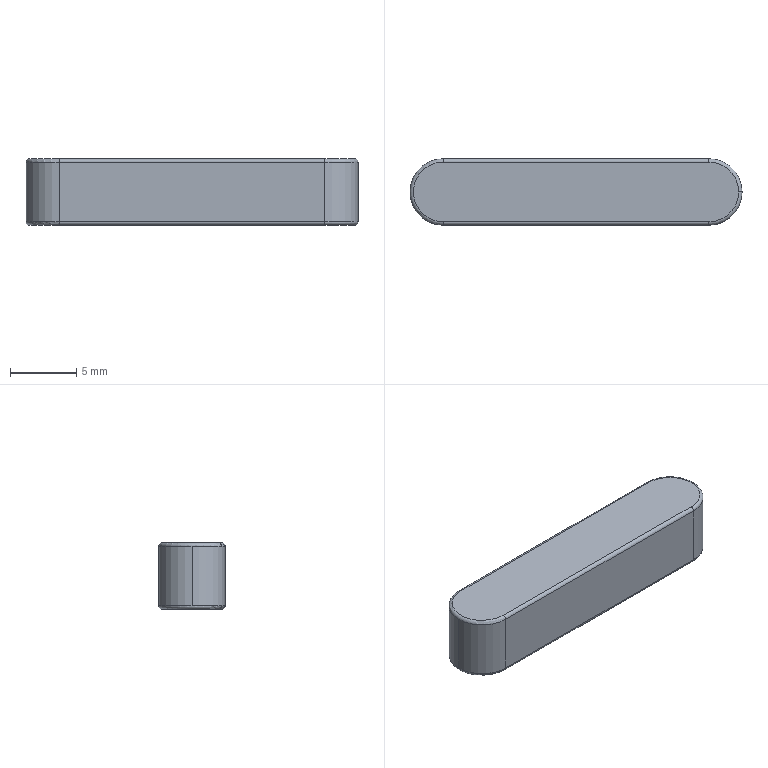Part | SolidWorks | features Extrusion 1, Fillet 1 | 1 solid | 17 faces | box 25 x 5 x 5 mm | volume 596.69 mm3 | cylinder 7 | torus 6 | plane 4 | commonest cylinder face diameters 0.5 x4 5 x3
STEP:
#1=CARTESIAN_POINT('',(12.25,0.,0.));
#2=VERTEX_POINT('',#1);
#3=CARTESIAN_POINT('',(10.,-2.25,0.));
#4=VERTEX_POINT('',#3);
#5=CARTESIAN_POINT('',(10.,0.,0.));
#6=DIRECTION('',(0.,0.,-1.));
#7=DIRECTION('',(1.,0.,0.));
#8=AXIS2_PLACEMENT_3D('',#5,#6,#7);
#9=CIRCLE('',#8,2.25);
#10=EDGE_CURVE('',#2,#4,#9,.T.);
#11=ORIENTED_EDGE('',*,*,#10,.F.);
#12=CARTESIAN_POINT('',(12.5,0.,0.25));
#13=VERTEX_POINT('',#12);
#14=CARTESIAN_POINT('',(12.25,0.,0.25));
#15=DIRECTION('',(0.,-1.,0.));
#16=DIRECTION('',(0.,0.,-1.));
#17=AXIS2_PLACEMENT_3D('',#14,#15,#16);
#18=CIRCLE('',#17,0.25);
#19=EDGE_CURVE('',#2,#13,#18,.T.);
#20=ORIENTED_EDGE('',*,*,#19,.T.);
#21=CARTESIAN_POINT('',(10.,-2.5,0.25));
#22=VERTEX_POINT('',#21);
#23=CARTESIAN_POINT('',(10.,0.,0.25));
#24=DIRECTION('',(0.,0.,1.));
#25=DIRECTION('',(1.,0.,0.));
#26=AXIS2_PLACEMENT_3D('',#23,#24,#25);
#27=CIRCLE('',#26,2.5);
#28=EDGE_CURVE('',#22,#13,#27,.T.);
#29=ORIENTED_EDGE('',*,*,#28,.F.);
#30=CARTESIAN_POINT('',(10.,-2.25,0.25));
#31=DIRECTION('',(1.,0.,0.));
#32=DIRECTION('',(0.,0.,-1.));
#33=AXIS2_PLACEMENT_3D('',#30,#31,#32);
#34=CIRCLE('',#33,0.25);
#35=EDGE_CURVE('',#22,#4,#34,.T.);
#36=ORIENTED_EDGE('',*,*,#35,.T.);
#37=EDGE_LOOP('',(#11,#20,#29,#36));
#38=FACE_OUTER_BOUND('',#37,.T.);
#39=CARTESIAN_POINT('',(10.,0.,0.25));
#40=DIRECTION('',(0.,0.,1.));
#41=DIRECTION('',(1.,0.,0.));
#42=AXIS2_PLACEMENT_3D('',#39,#40,#41);
#43=TOROIDAL_SURFACE('',#42,2.25,0.25);
#44=ADVANCED_FACE('',(#38),#43,.T.);
#45=CARTESIAN_POINT('',(12.5,0.,4.75));
#46=VERTEX_POINT('',#45);
#47=CARTESIAN_POINT('',(10.,-2.5,4.75));
#48=VERTEX_POINT('',#47);
#49=CARTESIAN_POINT('',(10.,0.,4.75));
#50=DIRECTION('',(0.,0.,-1.));
#51=DIRECTION('',(1.,0.,0.));
#52=AXIS2_PLACEMENT_3D('',#49,#50,#51);
#53=CIRCLE('',#52,2.5);
#54=EDGE_CURVE('',#46,#48,#53,.T.);
#55=ORIENTED_EDGE('',*,*,#54,.F.);
#56=CARTESIAN_POINT('',(12.25,0.,5.));
#57=VERTEX_POINT('',#56);
#58=CARTESIAN_POINT('',(12.25,0.,4.75));
#59=DIRECTION('',(0.,-1.,0.));
#60=DIRECTION('',(0.,0.,-1.));
#61=AXIS2_PLACEMENT_3D('',#58,#59,#60);
#62=CIRCLE('',#61,0.25);
#63=EDGE_CURVE('',#46,#57,#62,.T.);
#64=ORIENTED_EDGE('',*,*,#63,.T.);
#65=CARTESIAN_POINT('',(10.,-2.25,5.));
#66=VERTEX_POINT('',#65);
#67=CARTESIAN_POINT('',(10.,0.,5.));
#68=DIRECTION('',(0.,0.,1.));
#69=DIRECTION('',(1.,0.,0.));
#70=AXIS2_PLACEMENT_3D('',#67,#68,#69);
#71=CIRCLE('',#70,2.25);
#72=EDGE_CURVE('',#66,#57,#71,.T.);
#73=ORIENTED_EDGE('',*,*,#72,.F.);
#74=CARTESIAN_POINT('',(10.,-2.25,4.75));
#75=DIRECTION('',(1.,0.,0.));
#76=DIRECTION('',(0.,0.,-1.));
#77=AXIS2_PLACEMENT_3D('',#74,#75,#76);
#78=CIRCLE('',#77,0.25);
#79=EDGE_CURVE('',#66,#48,#78,.T.);
#80=ORIENTED_EDGE('',*,*,#79,.T.);
#81=EDGE_LOOP('',(#55,#64,#73,#80));
#82=FACE_OUTER_BOUND('',#81,.T.);
#83=CARTESIAN_POINT('',(10.,0.,4.75));
#84=DIRECTION('',(0.,0.,1.));
#85=DIRECTION('',(1.,0.,0.));
#86=AXIS2_PLACEMENT_3D('',#83,#84,#85);
#87=TOROIDAL_SURFACE('',#86,2.25,0.25);
#88=ADVANCED_FACE('',(#82),#87,.T.);
#89=CARTESIAN_POINT('',(-10.,-2.5,4.75));
#90=VERTEX_POINT('',#89);
#91=CARTESIAN_POINT('',(-12.5,0.,4.75));
#92=VERTEX_POINT('',#91);
#93=CARTESIAN_POINT('',(-10.,0.,4.75));
#94=DIRECTION('',(0.,0.,-1.));
#95=DIRECTION('',(1.,0.,0.));
#96=AXIS2_PLACEMENT_3D('',#93,#94,#95);
#97=CIRCLE('',#96,2.5);
#98=EDGE_CURVE('',#90,#92,#97,.T.);
#99=ORIENTED_EDGE('',*,*,#98,.T.);
#100=CARTESIAN_POINT('',(-12.5,0.,0.25));
#101=VERTEX_POINT('',#100);
#102=CARTESIAN_POINT('',(-12.5,0.,5.));
#103=DIRECTION('',(0.,0.,-1.));
#104=VECTOR('',#103,1000.);
#105=LINE('',#102,#104);
#106=EDGE_CURVE('',#92,#101,#105,.T.);
#107=ORIENTED_EDGE('',*,*,#106,.T.);
#108=CARTESIAN_POINT('',(-10.,-2.5,0.25));
#109=VERTEX_POINT('',#108);
#110=CARTESIAN_POINT('',(-10.,0.,0.25));
#111=DIRECTION('',(0.,0.,1.));
#112=DIRECTION('',(1.,0.,0.));
#113=AXIS2_PLACEMENT_3D('',#110,#111,#112);
#114=CIRCLE('',#113,2.5);
#115=EDGE_CURVE('',#101,#109,#114,.T.);
#116=ORIENTED_EDGE('',*,*,#115,.T.);
#117=CARTESIAN_POINT('',(-10.,-2.5,5.));
#118=DIRECTION('',(0.,0.,-1.));
#119=VECTOR('',#118,1000.);
#120=LINE('',#117,#119);
#121=EDGE_CURVE('',#90,#109,#120,.T.);
#122=ORIENTED_EDGE('',*,*,#121,.F.);
#123=EDGE_LOOP('',(#99,#107,#116,#122));
#124=FACE_OUTER_BOUND('',#123,.T.);
#125=CARTESIAN_POINT('',(-10.,0.,5.));
#126=DIRECTION('',(0.,0.,-1.));
#127=DIRECTION('',(-1.,0.,0.));
#128=AXIS2_PLACEMENT_3D('',#125,#126,#127);
#129=CYLINDRICAL_SURFACE('',#128,2.5);
#130=ADVANCED_FACE('',(#124),#129,.T.);
#131=ORIENTED_EDGE('',*,*,#106,.F.);
#132=CARTESIAN_POINT('',(-10.,2.5,4.75));
#133=VERTEX_POINT('',#132);
#134=CARTESIAN_POINT('',(-10.,0.,4.75));
#135=DIRECTION('',(0.,0.,-1.));
#136=DIRECTION('',(1.,0.,0.));
#137=AXIS2_PLACEMENT_3D('',#134,#135,#136);
#138=CIRCLE('',#137,2.5);
#139=EDGE_CURVE('',#92,#133,#138,.T.);
#140=ORIENTED_EDGE('',*,*,#139,.T.);
#141=CARTESIAN_POINT('',(-10.,2.5,0.25));
#142=VERTEX_POINT('',#141);
#143=CARTESIAN_POINT('',(-10.,2.5,5.));
#144=DIRECTION('',(0.,0.,-1.));
#145=VECTOR('',#144,1000.);
#146=LINE('',#143,#145);
#147=EDGE_CURVE('',#133,#142,#146,.T.);
#148=ORIENTED_EDGE('',*,*,#147,.T.);
#149=CARTESIAN_POINT('',(-10.,0.,0.25));
#150=DIRECTION('',(0.,0.,1.));
#151=DIRECTION('',(1.,0.,0.));
#152=AXIS2_PLACEMENT_3D('',#149,#150,#151);
#153=CIRCLE('',#152,2.5);
#154=EDGE_CURVE('',#142,#101,#153,.T.);
#155=ORIENTED_EDGE('',*,*,#154,.T.);
#156=EDGE_LOOP('',(#131,#140,#148,#155));
#157=FACE_OUTER_BOUND('',#156,.T.);
#158=CARTESIAN_POINT('',(-10.,0.,5.));
#159=DIRECTION('',(0.,0.,-1.));
#160=DIRECTION('',(-1.,0.,0.));
#161=AXIS2_PLACEMENT_3D('',#158,#159,#160);
#162=CYLINDRICAL_SURFACE('',#161,2.5);
#163=ADVANCED_FACE('',(#157),#162,.T.);
#164=CARTESIAN_POINT('',(10.,-2.5,5.));
#165=DIRECTION('',(0.,0.,-1.));
#166=VECTOR('',#165,1000.);
#167=LINE('',#164,#166);
#168=EDGE_CURVE('',#48,#22,#167,.T.);
#169=ORIENTED_EDGE('',*,*,#168,.F.);
#170=CARTESIAN_POINT('',(-10.,-2.5,4.75));
#171=DIRECTION('',(-1.,0.,0.));
#172=VECTOR('',#171,1000.);
#173=LINE('',#170,#172);
#174=EDGE_CURVE('',#48,#90,#173,.T.);
#175=ORIENTED_EDGE('',*,*,#174,.T.);
#176=ORIENTED_EDGE('',*,*,#121,.T.);
#177=CARTESIAN_POINT('',(-10.,-2.5,0.25));
#178=DIRECTION('',(1.,0.,0.));
#179=VECTOR('',#178,1000.);
#180=LINE('',#177,#179);
#181=EDGE_CURVE('',#109,#22,#180,.T.);
#182=ORIENTED_EDGE('',*,*,#181,.T.);
#183=EDGE_LOOP('',(#169,#175,#176,#182));
#184=FACE_OUTER_BOUND('',#183,.T.);
#185=CARTESIAN_POINT('',(-10.,-2.5,5.));
#186=DIRECTION('',(0.,1.,0.));
#187=DIRECTION('',(0.,0.,1.));
#188=AXIS2_PLACEMENT_3D('',#185,#186,#187);
#189=PLANE('',#188);
#190=ADVANCED_FACE('',(#184),#189,.F.);
#191=CARTESIAN_POINT('',(10.,2.5,4.75));
#192=VERTEX_POINT('',#191);
#193=CARTESIAN_POINT('',(10.,2.5,0.25));
#194=VERTEX_POINT('',#193);
#195=CARTESIAN_POINT('',(10.,2.5,5.));
#196=DIRECTION('',(0.,0.,-1.));
#197=VECTOR('',#196,1000.);
#198=LINE('',#195,#197);
#199=EDGE_CURVE('',#192,#194,#198,.T.);
#200=ORIENTED_EDGE('',*,*,#199,.F.);
#201=CARTESIAN_POINT('',(10.,0.,4.75));
#202=DIRECTION('',(0.,0.,-1.));
#203=DIRECTION('',(1.,0.,0.));
#204=AXIS2_PLACEMENT_3D('',#201,#202,#203);
#205=CIRCLE('',#204,2.5);
#206=EDGE_CURVE('',#192,#46,#205,.T.);
#207=ORIENTED_EDGE('',*,*,#206,.T.);
#208=ORIENTED_EDGE('',*,*,#54,.T.);
#209=ORIENTED_EDGE('',*,*,#168,.T.);
#210=ORIENTED_EDGE('',*,*,#28,.T.);
#211=CARTESIAN_POINT('',(10.,0.,0.25));
#212=DIRECTION('',(0.,0.,1.));
#213=DIRECTION('',(1.,0.,0.));
#214=AXIS2_PLACEMENT_3D('',#211,#212,#213);
#215=CIRCLE('',#214,2.5);
#216=EDGE_CURVE('',#13,#194,#215,.T.);
#217=ORIENTED_EDGE('',*,*,#216,.T.);
#218=EDGE_LOOP('',(#200,#207,#208,#209,#210,#217));
#219=FACE_OUTER_BOUND('',#218,.T.);
#220=CARTESIAN_POINT('',(10.,0.,5.));
#221=DIRECTION('',(0.,0.,-1.));
#222=DIRECTION('',(-1.,0.,0.));
#223=AXIS2_PLACEMENT_3D('',#220,#221,#222);
#224=CYLINDRICAL_SURFACE('',#223,2.5);
#225=ADVANCED_FACE('',(#219),#224,.T.);
#226=ORIENTED_EDGE('',*,*,#147,.F.);
#227=CARTESIAN_POINT('',(10.,2.5,4.75));
#228=DIRECTION('',(1.,0.,0.));
#229=VECTOR('',#228,1000.);
#230=LINE('',#227,#229);
#231=EDGE_CURVE('',#133,#192,#230,.T.);
#232=ORIENTED_EDGE('',*,*,#231,.T.);
#233=ORIENTED_EDGE('',*,*,#199,.T.);
#234=CARTESIAN_POINT('',(-10.,2.5,0.25));
#235=DIRECTION('',(-1.,0.,0.));
#236=VECTOR('',#235,1000.);
#237=LINE('',#234,#236);
#238=EDGE_CURVE('',#194,#142,#237,.T.);
#239=ORIENTED_EDGE('',*,*,#238,.T.);
#240=EDGE_LOOP('',(#226,#232,#233,#239));
#241=FACE_OUTER_BOUND('',#240,.T.);
#242=CARTESIAN_POINT('',(-10.,2.5,5.));
#243=DIRECTION('',(0.,-1.,0.));
#244=DIRECTION('',(0.,0.,-1.));
#245=AXIS2_PLACEMENT_3D('',#242,#243,#244);
#246=PLANE('',#245);
#247=ADVANCED_FACE('',(#241),#246,.F.);
#248=CARTESIAN_POINT('',(-10.,-2.25,5.));
#249=VERTEX_POINT('',#248);
#250=CARTESIAN_POINT('',(10.,-2.25,5.));
#251=DIRECTION('',(1.,0.,0.));
#252=VECTOR('',#251,1000.);
#253=LINE('',#250,#252);
#254=EDGE_CURVE('',#249,#66,#253,.T.);
#255=ORIENTED_EDGE('',*,*,#254,.T.);
#256=ORIENTED_EDGE('',*,*,#72,.T.);
#257=CARTESIAN_POINT('',(10.,2.25,5.));
#258=VERTEX_POINT('',#257);
#259=CARTESIAN_POINT('',(10.,0.,5.));
#260=DIRECTION('',(0.,0.,1.));
#261=DIRECTION('',(1.,0.,0.));
#262=AXIS2_PLACEMENT_3D('',#259,#260,#261);
#263=CIRCLE('',#262,2.25);
#264=EDGE_CURVE('',#57,#258,#263,.T.);
#265=ORIENTED_EDGE('',*,*,#264,.T.);
#266=CARTESIAN_POINT('',(-10.,2.25,5.));
#267=VERTEX_POINT('',#266);
#268=CARTESIAN_POINT('',(-10.,2.25,5.));
#269=DIRECTION('',(-1.,0.,0.));
#270=VECTOR('',#269,1000.);
#271=LINE('',#268,#270);
#272=EDGE_CURVE('',#258,#267,#271,.T.);
#273=ORIENTED_EDGE('',*,*,#272,.T.);
#274=CARTESIAN_POINT('',(-10.,0.,5.));
#275=DIRECTION('',(0.,0.,1.));
#276=DIRECTION('',(1.,0.,0.));
#277=AXIS2_PLACEMENT_3D('',#274,#275,#276);
#278=CIRCLE('',#277,2.25);
#279=EDGE_CURVE('',#267,#249,#278,.T.);
#280=ORIENTED_EDGE('',*,*,#279,.T.);
#281=EDGE_LOOP('',(#255,#256,#265,#273,#280));
#282=FACE_OUTER_BOUND('',#281,.T.);
#283=CARTESIAN_POINT('',(-10.,0.,5.));
#284=DIRECTION('',(0.,0.,1.));
#285=DIRECTION('',(1.,0.,0.));
#286=AXIS2_PLACEMENT_3D('',#283,#284,#285);
#287=PLANE('',#286);
#288=ADVANCED_FACE('',(#282),#287,.T.);
#289=CARTESIAN_POINT('',(-10.,2.25,0.));
#290=VERTEX_POINT('',#289);
#291=CARTESIAN_POINT('',(10.,2.25,0.));
#292=VERTEX_POINT('',#291);
#293=CARTESIAN_POINT('',(-10.,2.25,0.));
#294=DIRECTION('',(1.,0.,0.));
#295=VECTOR('',#294,1000.);
#296=LINE('',#293,#295);
#297=EDGE_CURVE('',#290,#292,#296,.T.);
#298=ORIENTED_EDGE('',*,*,#297,.T.);
#299=CARTESIAN_POINT('',(10.,0.,0.));
#300=DIRECTION('',(0.,0.,-1.));
#301=DIRECTION('',(1.,0.,0.));
#302=AXIS2_PLACEMENT_3D('',#299,#300,#301);
#303=CIRCLE('',#302,2.25);
#304=EDGE_CURVE('',#292,#2,#303,.T.);
#305=ORIENTED_EDGE('',*,*,#304,.T.);
#306=ORIENTED_EDGE('',*,*,#10,.T.);
#307=CARTESIAN_POINT('',(-10.,-2.25,0.));
#308=VERTEX_POINT('',#307);
#309=CARTESIAN_POINT('',(-10.,-2.25,0.));
#310=DIRECTION('',(-1.,0.,0.));
#311=VECTOR('',#310,1000.);
#312=LINE('',#309,#311);
#313=EDGE_CURVE('',#4,#308,#312,.T.);
#314=ORIENTED_EDGE('',*,*,#313,.T.);
#315=CARTESIAN_POINT('',(-10.,0.,0.));
#316=DIRECTION('',(0.,0.,-1.));
#317=DIRECTION('',(1.,0.,0.));
#318=AXIS2_PLACEMENT_3D('',#315,#316,#317);
#319=CIRCLE('',#318,2.25);
#320=EDGE_CURVE('',#308,#290,#319,.T.);
#321=ORIENTED_EDGE('',*,*,#320,.T.);
#322=EDGE_LOOP('',(#298,#305,#306,#314,#321));
#323=FACE_OUTER_BOUND('',#322,.T.);
#324=CARTESIAN_POINT('',(-10.,0.,0.));
#325=DIRECTION('',(0.,0.,1.));
#326=DIRECTION('',(1.,0.,0.));
#327=AXIS2_PLACEMENT_3D('',#324,#325,#326);
#328=PLANE('',#327);
#329=ADVANCED_FACE('',(#323),#328,.F.);
#330=CARTESIAN_POINT('',(-10.,2.25,4.75));
#331=DIRECTION('',(1.,0.,0.));
#332=DIRECTION('',(0.,0.,-1.));
#333=AXIS2_PLACEMENT_3D('',#330,#331,#332);
#334=CIRCLE('',#333,0.25);
#335=EDGE_CURVE('',#133,#267,#334,.T.);
#336=ORIENTED_EDGE('',*,*,#335,.F.);
#337=ORIENTED_EDGE('',*,*,#139,.F.);
#338=ORIENTED_EDGE('',*,*,#98,.F.);
#339=CARTESIAN_POINT('',(-10.,-2.25,4.75));
#340=DIRECTION('',(1.,0.,0.));
#341=DIRECTION('',(0.,0.,-1.));
#342=AXIS2_PLACEMENT_3D('',#339,#340,#341);
#343=CIRCLE('',#342,0.25);
#344=EDGE_CURVE('',#249,#90,#343,.T.);
#345=ORIENTED_EDGE('',*,*,#344,.F.);
#346=ORIENTED_EDGE('',*,*,#279,.F.);
#347=EDGE_LOOP('',(#336,#337,#338,#345,#346));
#348=FACE_OUTER_BOUND('',#347,.T.);
#349=CARTESIAN_POINT('',(-10.,0.,4.75));
#350=DIRECTION('',(0.,0.,1.));
#351=DIRECTION('',(1.,0.,0.));
#352=AXIS2_PLACEMENT_3D('',#349,#350,#351);
#353=TOROIDAL_SURFACE('',#352,2.25,0.25);
#354=ADVANCED_FACE('',(#348),#353,.T.);
#355=ORIENTED_EDGE('',*,*,#344,.T.);
#356=ORIENTED_EDGE('',*,*,#174,.F.);
#357=ORIENTED_EDGE('',*,*,#79,.F.);
#358=ORIENTED_EDGE('',*,*,#254,.F.);
#359=EDGE_LOOP('',(#355,#356,#357,#358));
#360=FACE_OUTER_BOUND('',#359,.T.);
#361=CARTESIAN_POINT('',(-10.,-2.25,4.75));
#362=DIRECTION('',(-1.,0.,0.));
#363=DIRECTION('',(0.,0.,1.));
#364=AXIS2_PLACEMENT_3D('',#361,#362,#363);
#365=CYLINDRICAL_SURFACE('',#364,0.25);
#366=ADVANCED_FACE('',(#360),#365,.T.);
#367=ORIENTED_EDGE('',*,*,#335,.T.);
#368=ORIENTED_EDGE('',*,*,#272,.F.);
#369=CARTESIAN_POINT('',(10.,2.25,4.75));
#370=DIRECTION('',(1.,0.,0.));
#371=DIRECTION('',(0.,0.,-1.));
#372=AXIS2_PLACEMENT_3D('',#369,#370,#371);
#373=CIRCLE('',#372,0.25);
#374=EDGE_CURVE('',#192,#258,#373,.T.);
#375=ORIENTED_EDGE('',*,*,#374,.F.);
#376=ORIENTED_EDGE('',*,*,#231,.F.);
#377=EDGE_LOOP('',(#367,#368,#375,#376));
#378=FACE_OUTER_BOUND('',#377,.T.);
#379=CARTESIAN_POINT('',(-10.,2.25,4.75));
#380=DIRECTION('',(1.,0.,0.));
#381=DIRECTION('',(0.,0.,-1.));
#382=AXIS2_PLACEMENT_3D('',#379,#380,#381);
#383=CYLINDRICAL_SURFACE('',#382,0.25);
#384=ADVANCED_FACE('',(#378),#383,.T.);
#385=ORIENTED_EDGE('',*,*,#63,.F.);
#386=ORIENTED_EDGE('',*,*,#206,.F.);
#387=ORIENTED_EDGE('',*,*,#374,.T.);
#388=ORIENTED_EDGE('',*,*,#264,.F.);
#389=EDGE_LOOP('',(#385,#386,#387,#388));
#390=FACE_OUTER_BOUND('',#389,.T.);
#391=CARTESIAN_POINT('',(10.,0.,4.75));
#392=DIRECTION('',(0.,0.,1.));
#393=DIRECTION('',(1.,0.,0.));
#394=AXIS2_PLACEMENT_3D('',#391,#392,#393);
#395=TOROIDAL_SURFACE('',#394,2.25,0.25);
#396=ADVANCED_FACE('',(#390),#395,.T.);
#397=CARTESIAN_POINT('',(-10.,2.25,0.25));
#398=DIRECTION('',(1.,0.,0.));
#399=DIRECTION('',(0.,0.,-1.));
#400=AXIS2_PLACEMENT_3D('',#397,#398,#399);
#401=CIRCLE('',#400,0.25);
#402=EDGE_CURVE('',#290,#142,#401,.T.);
#403=ORIENTED_EDGE('',*,*,#402,.F.);
#404=ORIENTED_EDGE('',*,*,#320,.F.);
#405=CARTESIAN_POINT('',(-10.,-2.25,0.25));
#406=DIRECTION('',(1.,0.,0.));
#407=DIRECTION('',(0.,0.,-1.));
#408=AXIS2_PLACEMENT_3D('',#405,#406,#407);
#409=CIRCLE('',#408,0.25);
#410=EDGE_CURVE('',#109,#308,#409,.T.);
#411=ORIENTED_EDGE('',*,*,#410,.F.);
#412=ORIENTED_EDGE('',*,*,#115,.F.);
#413=ORIENTED_EDGE('',*,*,#154,.F.);
#414=EDGE_LOOP('',(#403,#404,#411,#412,#413));
#415=FACE_OUTER_BOUND('',#414,.T.);
#416=CARTESIAN_POINT('',(-10.,0.,0.25));
#417=DIRECTION('',(0.,0.,1.));
#418=DIRECTION('',(1.,0.,0.));
#419=AXIS2_PLACEMENT_3D('',#416,#417,#418);
#420=TOROIDAL_SURFACE('',#419,2.25,0.25);
#421=ADVANCED_FACE('',(#415),#420,.T.);
#422=ORIENTED_EDGE('',*,*,#410,.T.);
#423=ORIENTED_EDGE('',*,*,#313,.F.);
#424=ORIENTED_EDGE('',*,*,#35,.F.);
#425=ORIENTED_EDGE('',*,*,#181,.F.);
#426=EDGE_LOOP('',(#422,#423,#424,#425));
#427=FACE_OUTER_BOUND('',#426,.T.);
#428=CARTESIAN_POINT('',(-10.,-2.25,0.25));
#429=DIRECTION('',(1.,0.,0.));
#430=DIRECTION('',(0.,0.,-1.));
#431=AXIS2_PLACEMENT_3D('',#428,#429,#430);
#432=CYLINDRICAL_SURFACE('',#431,0.25);
#433=ADVANCED_FACE('',(#427),#432,.T.);
#434=ORIENTED_EDGE('',*,*,#402,.T.);
#435=ORIENTED_EDGE('',*,*,#238,.F.);
#436=CARTESIAN_POINT('',(10.,2.25,0.25));
#437=DIRECTION('',(1.,0.,0.));
#438=DIRECTION('',(0.,0.,-1.));
#439=AXIS2_PLACEMENT_3D('',#436,#437,#438);
#440=CIRCLE('',#439,0.25);
#441=EDGE_CURVE('',#292,#194,#440,.T.);
#442=ORIENTED_EDGE('',*,*,#441,.F.);
#443=ORIENTED_EDGE('',*,*,#297,.F.);
#444=EDGE_LOOP('',(#434,#435,#442,#443));
#445=FACE_OUTER_BOUND('',#444,.T.);
#446=CARTESIAN_POINT('',(-10.,2.25,0.25));
#447=DIRECTION('',(-1.,0.,0.));
#448=DIRECTION('',(0.,0.,1.));
#449=AXIS2_PLACEMENT_3D('',#446,#447,#448);
#450=CYLINDRICAL_SURFACE('',#449,0.25);
#451=ADVANCED_FACE('',(#445),#450,.T.);
#452=ORIENTED_EDGE('',*,*,#19,.F.);
#453=ORIENTED_EDGE('',*,*,#304,.F.);
#454=ORIENTED_EDGE('',*,*,#441,.T.);
#455=ORIENTED_EDGE('',*,*,#216,.F.);
#456=EDGE_LOOP('',(#452,#453,#454,#455));
#457=FACE_OUTER_BOUND('',#456,.T.);
#458=CARTESIAN_POINT('',(10.,0.,0.25));
#459=DIRECTION('',(0.,0.,1.));
#460=DIRECTION('',(1.,0.,0.));
#461=AXIS2_PLACEMENT_3D('',#458,#459,#460);
#462=TOROIDAL_SURFACE('',#461,2.25,0.25);
#463=ADVANCED_FACE('',(#457),#462,.T.);
#464=CLOSED_SHELL('',(#44,#88,#130,#163,#190,#225,#247,#288,#329,#354,#366,#384,#396,#421,#433,#451,#463));
#465=MANIFOLD_SOLID_BREP('',#464);
#466=CARTESIAN_POINT('',(0.,0.,0.));
#467=DIRECTION('',(0.,0.,1.));
#468=DIRECTION('',(1.,0.,0.));
#469=AXIS2_PLACEMENT_3D('',#466,#467,#468);
#470=(LENGTH_UNIT()NAMED_UNIT(*)SI_UNIT(.MILLI.,.METRE.));
#471=UNCERTAINTY_MEASURE_WITH_UNIT(LENGTH_MEASURE(0.00001),#470,'','');
#472=(NAMED_UNIT(*)PLANE_ANGLE_UNIT()SI_UNIT($,.RADIAN.));
#473=(NAMED_UNIT(*)SI_UNIT($,.STERADIAN.)SOLID_ANGLE_UNIT());
#474=(GEOMETRIC_REPRESENTATION_CONTEXT(3)GLOBAL_UNCERTAINTY_ASSIGNED_CONTEXT((#471))GLOBAL_UNIT_ASSIGNED_CONTEXT((#470,#472,#473))REPRESENTATION_CONTEXT('',''));
#475=ADVANCED_BREP_SHAPE_REPRESENTATION('',(#465,#469),#474);